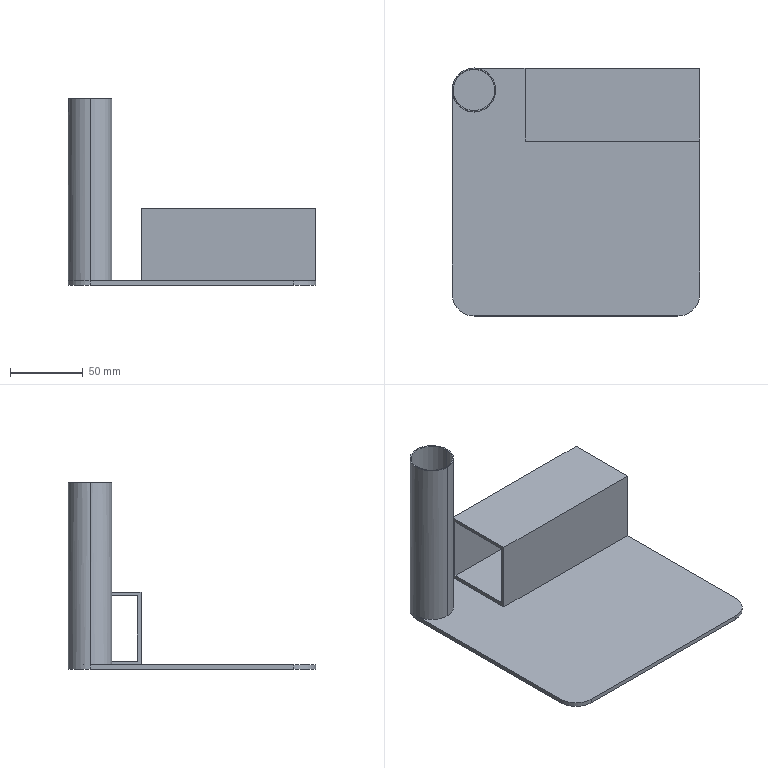Part | STEP file | Component1 | 1 solid | 23 faces | box 170 x 170 x 128 mm | volume 151175 mm3 | plane 16 | cylinder 7 | commonest cylinder face diameters 30 x5 28.6 x2
STEP:
#1=CARTESIAN_POINT('',(29.3,155.,2.));
#2=VERTEX_POINT('',#1);
#3=CARTESIAN_POINT('',(0.7,155.,2.));
#4=VERTEX_POINT('',#3);
#5=CARTESIAN_POINT('',(15.,155.,2.));
#6=DIRECTION('',(0.,0.,1.));
#7=DIRECTION('',(-1.,0.,0.));
#8=AXIS2_PLACEMENT_3D('',#5,#6,#7);
#9=CIRCLE('',#8,14.3);
#10=EDGE_CURVE('',#2,#4,#9,.T.);
#11=ORIENTED_EDGE('',*,*,#10,.F.);
#12=CARTESIAN_POINT('',(29.3,155.,127.));
#13=VERTEX_POINT('',#12);
#14=CARTESIAN_POINT('',(29.3,155.,2.));
#15=DIRECTION('',(0.,0.,1.));
#16=VECTOR('',#15,1000.);
#17=LINE('',#14,#16);
#18=EDGE_CURVE('',#2,#13,#17,.T.);
#19=ORIENTED_EDGE('',*,*,#18,.T.);
#20=CARTESIAN_POINT('',(0.7,155.,127.));
#21=VERTEX_POINT('',#20);
#22=CARTESIAN_POINT('',(15.,155.,127.));
#23=DIRECTION('',(0.,0.,-1.));
#24=DIRECTION('',(-1.,0.,0.));
#25=AXIS2_PLACEMENT_3D('',#22,#23,#24);
#26=CIRCLE('',#25,14.3);
#27=EDGE_CURVE('',#21,#13,#26,.T.);
#28=ORIENTED_EDGE('',*,*,#27,.F.);
#29=CARTESIAN_POINT('',(0.7,155.,2.));
#30=DIRECTION('',(0.,0.,1.));
#31=VECTOR('',#30,1000.);
#32=LINE('',#29,#31);
#33=EDGE_CURVE('',#4,#21,#32,.T.);
#34=ORIENTED_EDGE('',*,*,#33,.F.);
#35=EDGE_LOOP('',(#11,#19,#28,#34));
#36=FACE_OUTER_BOUND('',#35,.T.);
#37=CARTESIAN_POINT('',(15.,155.,2.));
#38=DIRECTION('',(0.,0.,1.));
#39=DIRECTION('',(-1.,0.,0.));
#40=AXIS2_PLACEMENT_3D('',#37,#38,#39);
#41=CYLINDRICAL_SURFACE('',#40,14.3);
#42=ADVANCED_FACE('',(#36),#41,.F.);
#43=CARTESIAN_POINT('',(15.,140.,2.));
#44=VERTEX_POINT('',#43);
#45=CARTESIAN_POINT('',(0.,155.,2.));
#46=VERTEX_POINT('',#45);
#47=CARTESIAN_POINT('',(15.,155.,2.));
#48=DIRECTION('',(0.,0.,-1.));
#49=DIRECTION('',(-1.,0.,0.));
#50=AXIS2_PLACEMENT_3D('',#47,#48,#49);
#51=CIRCLE('',#50,15.);
#52=EDGE_CURVE('',#44,#46,#51,.T.);
#53=ORIENTED_EDGE('',*,*,#52,.F.);
#54=CARTESIAN_POINT('',(15.,140.,127.));
#55=VERTEX_POINT('',#54);
#56=CARTESIAN_POINT('',(15.,140.,0.));
#57=DIRECTION('',(0.,0.,1.));
#58=VECTOR('',#57,1000.);
#59=LINE('',#56,#58);
#60=EDGE_CURVE('',#44,#55,#59,.T.);
#61=ORIENTED_EDGE('',*,*,#60,.T.);
#62=CARTESIAN_POINT('',(15.,170.,127.));
#63=VERTEX_POINT('',#62);
#64=CARTESIAN_POINT('',(15.,155.,127.));
#65=DIRECTION('',(0.,0.,1.));
#66=DIRECTION('',(-1.,0.,0.));
#67=AXIS2_PLACEMENT_3D('',#64,#65,#66);
#68=CIRCLE('',#67,15.);
#69=EDGE_CURVE('',#63,#55,#68,.T.);
#70=ORIENTED_EDGE('',*,*,#69,.F.);
#71=CARTESIAN_POINT('',(15.,170.,2.));
#72=VERTEX_POINT('',#71);
#73=CARTESIAN_POINT('',(15.,170.,0.));
#74=DIRECTION('',(0.,0.,1.));
#75=VECTOR('',#74,1000.);
#76=LINE('',#73,#75);
#77=EDGE_CURVE('',#72,#63,#76,.T.);
#78=ORIENTED_EDGE('',*,*,#77,.F.);
#79=CARTESIAN_POINT('',(15.,170.,-1.));
#80=VERTEX_POINT('',#79);
#81=CARTESIAN_POINT('',(15.,170.,0.));
#82=DIRECTION('',(0.,0.,-1.));
#83=VECTOR('',#82,1000.);
#84=LINE('',#81,#83);
#85=EDGE_CURVE('',#72,#80,#84,.T.);
#86=ORIENTED_EDGE('',*,*,#85,.T.);
#87=CARTESIAN_POINT('',(0.,155.,-1.));
#88=VERTEX_POINT('',#87);
#89=CARTESIAN_POINT('',(15.,155.,-1.));
#90=DIRECTION('',(0.,0.,-1.));
#91=DIRECTION('',(0.,1.,0.));
#92=AXIS2_PLACEMENT_3D('',#89,#90,#91);
#93=CIRCLE('',#92,15.);
#94=EDGE_CURVE('',#88,#80,#93,.T.);
#95=ORIENTED_EDGE('',*,*,#94,.F.);
#96=CARTESIAN_POINT('',(0.,155.,0.));
#97=DIRECTION('',(0.,0.,1.));
#98=VECTOR('',#97,1000.);
#99=LINE('',#96,#98);
#100=EDGE_CURVE('',#88,#46,#99,.T.);
#101=ORIENTED_EDGE('',*,*,#100,.T.);
#102=EDGE_LOOP('',(#53,#61,#70,#78,#86,#95,#101));
#103=FACE_OUTER_BOUND('',#102,.T.);
#104=CARTESIAN_POINT('',(15.,155.,0.));
#105=DIRECTION('',(0.,0.,1.));
#106=DIRECTION('',(0.,1.,0.));
#107=AXIS2_PLACEMENT_3D('',#104,#105,#106);
#108=CYLINDRICAL_SURFACE('',#107,15.);
#109=ADVANCED_FACE('',(#103),#108,.T.);
#110=CARTESIAN_POINT('',(15.,155.,2.));
#111=DIRECTION('',(0.,0.,1.));
#112=DIRECTION('',(-1.,0.,0.));
#113=AXIS2_PLACEMENT_3D('',#110,#111,#112);
#114=CIRCLE('',#113,14.3);
#115=EDGE_CURVE('',#4,#2,#114,.T.);
#116=ORIENTED_EDGE('',*,*,#115,.T.);
#117=ORIENTED_EDGE('',*,*,#10,.T.);
#118=EDGE_LOOP('',(#116,#117));
#119=FACE_OUTER_BOUND('',#118,.T.);
#120=CARTESIAN_POINT('',(85.,85.,2.));
#121=DIRECTION('',(0.,0.,1.));
#122=DIRECTION('',(1.,0.,0.));
#123=AXIS2_PLACEMENT_3D('',#120,#121,#122);
#124=PLANE('',#123);
#125=ADVANCED_FACE('',(#119),#124,.T.);
#126=ORIENTED_EDGE('',*,*,#60,.F.);
#127=CARTESIAN_POINT('',(15.,155.,2.));
#128=DIRECTION('',(0.,0.,-1.));
#129=DIRECTION('',(-1.,0.,0.));
#130=AXIS2_PLACEMENT_3D('',#127,#128,#129);
#131=CIRCLE('',#130,15.);
#132=EDGE_CURVE('',#72,#44,#131,.T.);
#133=ORIENTED_EDGE('',*,*,#132,.F.);
#134=ORIENTED_EDGE('',*,*,#77,.T.);
#135=CARTESIAN_POINT('',(15.,155.,127.));
#136=DIRECTION('',(0.,0.,1.));
#137=DIRECTION('',(-1.,0.,0.));
#138=AXIS2_PLACEMENT_3D('',#135,#136,#137);
#139=CIRCLE('',#138,15.);
#140=EDGE_CURVE('',#55,#63,#139,.T.);
#141=ORIENTED_EDGE('',*,*,#140,.F.);
#142=EDGE_LOOP('',(#126,#133,#134,#141));
#143=FACE_OUTER_BOUND('',#142,.T.);
#144=CARTESIAN_POINT('',(15.,155.,0.));
#145=DIRECTION('',(0.,0.,1.));
#146=DIRECTION('',(0.,1.,0.));
#147=AXIS2_PLACEMENT_3D('',#144,#145,#146);
#148=CYLINDRICAL_SURFACE('',#147,15.);
#149=ADVANCED_FACE('',(#143),#148,.T.);
#150=CARTESIAN_POINT('',(0.,15.,-1.));
#151=VERTEX_POINT('',#150);
#152=CARTESIAN_POINT('',(0.,15.,2.));
#153=VERTEX_POINT('',#152);
#154=CARTESIAN_POINT('',(0.,15.,0.));
#155=DIRECTION('',(0.,0.,1.));
#156=VECTOR('',#155,1000.);
#157=LINE('',#154,#156);
#158=EDGE_CURVE('',#151,#153,#157,.T.);
#159=ORIENTED_EDGE('',*,*,#158,.T.);
#160=CARTESIAN_POINT('',(0.,155.,2.));
#161=DIRECTION('',(0.,-1.,0.));
#162=VECTOR('',#161,1000.);
#163=LINE('',#160,#162);
#164=EDGE_CURVE('',#46,#153,#163,.T.);
#165=ORIENTED_EDGE('',*,*,#164,.F.);
#166=ORIENTED_EDGE('',*,*,#100,.F.);
#167=CARTESIAN_POINT('',(0.,155.,-1.));
#168=DIRECTION('',(0.,1.,0.));
#169=VECTOR('',#168,1000.);
#170=LINE('',#167,#169);
#171=EDGE_CURVE('',#151,#88,#170,.T.);
#172=ORIENTED_EDGE('',*,*,#171,.F.);
#173=EDGE_LOOP('',(#159,#165,#166,#172));
#174=FACE_OUTER_BOUND('',#173,.T.);
#175=CARTESIAN_POINT('',(0.,155.,0.));
#176=DIRECTION('',(-1.,0.,0.));
#177=DIRECTION('',(0.,1.,0.));
#178=AXIS2_PLACEMENT_3D('',#175,#176,#177);
#179=PLANE('',#178);
#180=ADVANCED_FACE('',(#174),#179,.T.);
#181=CARTESIAN_POINT('',(15.,0.,-1.));
#182=VERTEX_POINT('',#181);
#183=CARTESIAN_POINT('',(15.,0.,2.));
#184=VERTEX_POINT('',#183);
#185=CARTESIAN_POINT('',(15.,0.,0.));
#186=DIRECTION('',(0.,0.,1.));
#187=VECTOR('',#186,1000.);
#188=LINE('',#185,#187);
#189=EDGE_CURVE('',#182,#184,#188,.T.);
#190=ORIENTED_EDGE('',*,*,#189,.T.);
#191=CARTESIAN_POINT('',(15.,15.,2.));
#192=DIRECTION('',(0.,0.,1.));
#193=DIRECTION('',(-1.,0.,0.));
#194=AXIS2_PLACEMENT_3D('',#191,#192,#193);
#195=CIRCLE('',#194,15.);
#196=EDGE_CURVE('',#153,#184,#195,.T.);
#197=ORIENTED_EDGE('',*,*,#196,.F.);
#198=ORIENTED_EDGE('',*,*,#158,.F.);
#199=CARTESIAN_POINT('',(15.,15.,-1.));
#200=DIRECTION('',(0.,0.,-1.));
#201=DIRECTION('',(-1.,0.,0.));
#202=AXIS2_PLACEMENT_3D('',#199,#200,#201);
#203=CIRCLE('',#202,15.);
#204=EDGE_CURVE('',#182,#151,#203,.T.);
#205=ORIENTED_EDGE('',*,*,#204,.F.);
#206=EDGE_LOOP('',(#190,#197,#198,#205));
#207=FACE_OUTER_BOUND('',#206,.T.);
#208=CARTESIAN_POINT('',(15.,15.,0.));
#209=DIRECTION('',(0.,0.,1.));
#210=DIRECTION('',(-1.,0.,0.));
#211=AXIS2_PLACEMENT_3D('',#208,#209,#210);
#212=CYLINDRICAL_SURFACE('',#211,15.);
#213=ADVANCED_FACE('',(#207),#212,.T.);
#214=CARTESIAN_POINT('',(155.,0.,-1.));
#215=VERTEX_POINT('',#214);
#216=CARTESIAN_POINT('',(155.,0.,2.));
#217=VERTEX_POINT('',#216);
#218=CARTESIAN_POINT('',(155.,0.,0.));
#219=DIRECTION('',(0.,0.,1.));
#220=VECTOR('',#219,1000.);
#221=LINE('',#218,#220);
#222=EDGE_CURVE('',#215,#217,#221,.T.);
#223=ORIENTED_EDGE('',*,*,#222,.T.);
#224=CARTESIAN_POINT('',(15.,0.,2.));
#225=DIRECTION('',(1.,0.,0.));
#226=VECTOR('',#225,1000.);
#227=LINE('',#224,#226);
#228=EDGE_CURVE('',#184,#217,#227,.T.);
#229=ORIENTED_EDGE('',*,*,#228,.F.);
#230=ORIENTED_EDGE('',*,*,#189,.F.);
#231=CARTESIAN_POINT('',(15.,0.,-1.));
#232=DIRECTION('',(-1.,0.,0.));
#233=VECTOR('',#232,1000.);
#234=LINE('',#231,#233);
#235=EDGE_CURVE('',#215,#182,#234,.T.);
#236=ORIENTED_EDGE('',*,*,#235,.F.);
#237=EDGE_LOOP('',(#223,#229,#230,#236));
#238=FACE_OUTER_BOUND('',#237,.T.);
#239=CARTESIAN_POINT('',(15.,0.,0.));
#240=DIRECTION('',(0.,-1.,0.));
#241=DIRECTION('',(0.,0.,-1.));
#242=AXIS2_PLACEMENT_3D('',#239,#240,#241);
#243=PLANE('',#242);
#244=ADVANCED_FACE('',(#238),#243,.T.);
#245=CARTESIAN_POINT('',(170.,15.,-1.));
#246=VERTEX_POINT('',#245);
#247=CARTESIAN_POINT('',(170.,15.,2.));
#248=VERTEX_POINT('',#247);
#249=CARTESIAN_POINT('',(170.,15.,0.));
#250=DIRECTION('',(0.,0.,1.));
#251=VECTOR('',#250,1000.);
#252=LINE('',#249,#251);
#253=EDGE_CURVE('',#246,#248,#252,.T.);
#254=ORIENTED_EDGE('',*,*,#253,.T.);
#255=CARTESIAN_POINT('',(155.,15.,2.));
#256=DIRECTION('',(0.,0.,1.));
#257=DIRECTION('',(0.,-1.,0.));
#258=AXIS2_PLACEMENT_3D('',#255,#256,#257);
#259=CIRCLE('',#258,15.);
#260=EDGE_CURVE('',#217,#248,#259,.T.);
#261=ORIENTED_EDGE('',*,*,#260,.F.);
#262=ORIENTED_EDGE('',*,*,#222,.F.);
#263=CARTESIAN_POINT('',(155.,15.,-1.));
#264=DIRECTION('',(0.,0.,-1.));
#265=DIRECTION('',(0.,-1.,0.));
#266=AXIS2_PLACEMENT_3D('',#263,#264,#265);
#267=CIRCLE('',#266,15.);
#268=EDGE_CURVE('',#246,#215,#267,.T.);
#269=ORIENTED_EDGE('',*,*,#268,.F.);
#270=EDGE_LOOP('',(#254,#261,#262,#269));
#271=FACE_OUTER_BOUND('',#270,.T.);
#272=CARTESIAN_POINT('',(155.,15.,0.));
#273=DIRECTION('',(0.,0.,1.));
#274=DIRECTION('',(0.,-1.,0.));
#275=AXIS2_PLACEMENT_3D('',#272,#273,#274);
#276=CYLINDRICAL_SURFACE('',#275,15.);
#277=ADVANCED_FACE('',(#271),#276,.T.);
#278=CARTESIAN_POINT('',(170.,122.5,49.5));
#279=VERTEX_POINT('',#278);
#280=CARTESIAN_POINT('',(170.,167.5,49.5));
#281=VERTEX_POINT('',#280);
#282=CARTESIAN_POINT('',(170.,122.5,49.5));
#283=DIRECTION('',(0.,1.,0.));
#284=VECTOR('',#283,1000.);
#285=LINE('',#282,#284);
#286=EDGE_CURVE('',#279,#281,#285,.T.);
#287=ORIENTED_EDGE('',*,*,#286,.T.);
#288=CARTESIAN_POINT('',(170.,167.5,4.5));
#289=VERTEX_POINT('',#288);
#290=CARTESIAN_POINT('',(170.,167.5,49.5));
#291=DIRECTION('',(0.,0.,-1.));
#292=VECTOR('',#291,1000.);
#293=LINE('',#290,#292);
#294=EDGE_CURVE('',#281,#289,#293,.T.);
#295=ORIENTED_EDGE('',*,*,#294,.T.);
#296=CARTESIAN_POINT('',(170.,122.5,4.5));
#297=VERTEX_POINT('',#296);
#298=CARTESIAN_POINT('',(170.,167.5,4.5));
#299=DIRECTION('',(0.,-1.,0.));
#300=VECTOR('',#299,1000.);
#301=LINE('',#298,#300);
#302=EDGE_CURVE('',#289,#297,#301,.T.);
#303=ORIENTED_EDGE('',*,*,#302,.T.);
#304=CARTESIAN_POINT('',(170.,122.5,4.5));
#305=DIRECTION('',(0.,0.,1.));
#306=VECTOR('',#305,1000.);
#307=LINE('',#304,#306);
#308=EDGE_CURVE('',#297,#279,#307,.T.);
#309=ORIENTED_EDGE('',*,*,#308,.T.);
#310=EDGE_LOOP('',(#287,#295,#303,#309));
#311=FACE_BOUND('',#310,.T.);
#312=CARTESIAN_POINT('',(170.,155.,-1.));
#313=VERTEX_POINT('',#312);
#314=CARTESIAN_POINT('',(170.,155.,2.));
#315=VERTEX_POINT('',#314);
#316=CARTESIAN_POINT('',(170.,155.,0.));
#317=DIRECTION('',(0.,0.,1.));
#318=VECTOR('',#317,1000.);
#319=LINE('',#316,#318);
#320=EDGE_CURVE('',#313,#315,#319,.T.);
#321=ORIENTED_EDGE('',*,*,#320,.T.);
#322=CARTESIAN_POINT('',(170.,170.,2.));
#323=VERTEX_POINT('',#322);
#324=CARTESIAN_POINT('',(170.,170.,2.));
#325=DIRECTION('',(0.,-1.,0.));
#326=VECTOR('',#325,1000.);
#327=LINE('',#324,#326);
#328=EDGE_CURVE('',#323,#315,#327,.T.);
#329=ORIENTED_EDGE('',*,*,#328,.F.);
#330=CARTESIAN_POINT('',(170.,170.,52.));
#331=VERTEX_POINT('',#330);
#332=CARTESIAN_POINT('',(170.,170.,52.));
#333=DIRECTION('',(0.,0.,-1.));
#334=VECTOR('',#333,1000.);
#335=LINE('',#332,#334);
#336=EDGE_CURVE('',#331,#323,#335,.T.);
#337=ORIENTED_EDGE('',*,*,#336,.F.);
#338=CARTESIAN_POINT('',(170.,120.,52.));
#339=VERTEX_POINT('',#338);
#340=CARTESIAN_POINT('',(170.,120.,52.));
#341=DIRECTION('',(0.,1.,0.));
#342=VECTOR('',#341,1000.);
#343=LINE('',#340,#342);
#344=EDGE_CURVE('',#339,#331,#343,.T.);
#345=ORIENTED_EDGE('',*,*,#344,.F.);
#346=CARTESIAN_POINT('',(170.,120.,2.));
#347=VERTEX_POINT('',#346);
#348=CARTESIAN_POINT('',(170.,120.,2.));
#349=DIRECTION('',(0.,0.,1.));
#350=VECTOR('',#349,1000.);
#351=LINE('',#348,#350);
#352=EDGE_CURVE('',#347,#339,#351,.T.);
#353=ORIENTED_EDGE('',*,*,#352,.F.);
#354=CARTESIAN_POINT('',(170.,15.,2.));
#355=DIRECTION('',(0.,1.,0.));
#356=VECTOR('',#355,1000.);
#357=LINE('',#354,#356);
#358=EDGE_CURVE('',#248,#347,#357,.T.);
#359=ORIENTED_EDGE('',*,*,#358,.F.);
#360=ORIENTED_EDGE('',*,*,#253,.F.);
#361=CARTESIAN_POINT('',(170.,15.,-1.));
#362=DIRECTION('',(0.,-1.,0.));
#363=VECTOR('',#362,1000.);
#364=LINE('',#361,#363);
#365=EDGE_CURVE('',#313,#246,#364,.T.);
#366=ORIENTED_EDGE('',*,*,#365,.F.);
#367=EDGE_LOOP('',(#321,#329,#337,#345,#353,#359,#360,#366));
#368=FACE_OUTER_BOUND('',#367,.T.);
#369=CARTESIAN_POINT('',(170.,15.,0.));
#370=DIRECTION('',(1.,0.,0.));
#371=DIRECTION('',(0.,1.,0.));
#372=AXIS2_PLACEMENT_3D('',#369,#370,#371);
#373=PLANE('',#372);
#374=ADVANCED_FACE('',(#311,#368),#373,.T.);
#375=CARTESIAN_POINT('',(155.,170.,-1.));
#376=VERTEX_POINT('',#375);
#377=CARTESIAN_POINT('',(155.,170.,2.));
#378=VERTEX_POINT('',#377);
#379=CARTESIAN_POINT('',(155.,170.,0.));
#380=DIRECTION('',(0.,0.,1.));
#381=VECTOR('',#380,1000.);
#382=LINE('',#379,#381);
#383=EDGE_CURVE('',#376,#378,#382,.T.);
#384=ORIENTED_EDGE('',*,*,#383,.T.);
#385=CARTESIAN_POINT('',(155.,155.,2.));
#386=DIRECTION('',(0.,0.,1.));
#387=DIRECTION('',(1.,0.,0.));
#388=AXIS2_PLACEMENT_3D('',#385,#386,#387);
#389=CIRCLE('',#388,15.);
#390=EDGE_CURVE('',#315,#378,#389,.T.);
#391=ORIENTED_EDGE('',*,*,#390,.F.);
#392=ORIENTED_EDGE('',*,*,#320,.F.);
#393=CARTESIAN_POINT('',(155.,155.,-1.));
#394=DIRECTION('',(0.,0.,-1.));
#395=DIRECTION('',(1.,0.,0.));
#396=AXIS2_PLACEMENT_3D('',#393,#394,#395);
#397=CIRCLE('',#396,15.);
#398=EDGE_CURVE('',#376,#313,#397,.T.);
#399=ORIENTED_EDGE('',*,*,#398,.F.);
#400=EDGE_LOOP('',(#384,#391,#392,#399));
#401=FACE_OUTER_BOUND('',#400,.T.);
#402=CARTESIAN_POINT('',(155.,155.,0.));
#403=DIRECTION('',(0.,0.,1.));
#404=DIRECTION('',(1.,0.,0.));
#405=AXIS2_PLACEMENT_3D('',#402,#403,#404);
#406=CYLINDRICAL_SURFACE('',#405,15.);
#407=ADVANCED_FACE('',(#401),#406,.T.);
#408=ORIENTED_EDGE('',*,*,#85,.F.);
#409=CARTESIAN_POINT('',(50.,170.,2.));
#410=VERTEX_POINT('',#409);
#411=CARTESIAN_POINT('',(155.,170.,2.));
#412=DIRECTION('',(-1.,0.,0.));
#413=VECTOR('',#412,1000.);
#414=LINE('',#411,#413);
#415=EDGE_CURVE('',#410,#72,#414,.T.);
#416=ORIENTED_EDGE('',*,*,#415,.F.);
#417=CARTESIAN_POINT('',(50.,170.,52.));
#418=VERTEX_POINT('',#417);
#419=CARTESIAN_POINT('',(50.,170.,52.));
#420=DIRECTION('',(0.,0.,-1.));
#421=VECTOR('',#420,1000.);
#422=LINE('',#419,#421);
#423=EDGE_CURVE('',#418,#410,#422,.T.);
#424=ORIENTED_EDGE('',*,*,#423,.F.);
#425=CARTESIAN_POINT('',(170.,170.,52.));
#426=DIRECTION('',(-1.,0.,0.));
#427=VECTOR('',#426,1000.);
#428=LINE('',#425,#427);
#429=EDGE_CURVE('',#331,#418,#428,.T.);
#430=ORIENTED_EDGE('',*,*,#429,.F.);
#431=ORIENTED_EDGE('',*,*,#336,.T.);
#432=CARTESIAN_POINT('',(170.,170.,2.));
#433=DIRECTION('',(-1.,0.,0.));
#434=VECTOR('',#433,1000.);
#435=LINE('',#432,#434);
#436=EDGE_CURVE('',#323,#378,#435,.T.);
#437=ORIENTED_EDGE('',*,*,#436,.T.);
#438=ORIENTED_EDGE('',*,*,#383,.F.);
#439=CARTESIAN_POINT('',(155.,170.,-1.));
#440=DIRECTION('',(1.,0.,0.));
#441=VECTOR('',#440,1000.);
#442=LINE('',#439,#441);
#443=EDGE_CURVE('',#80,#376,#442,.T.);
#444=ORIENTED_EDGE('',*,*,#443,.F.);
#445=EDGE_LOOP('',(#408,#416,#424,#430,#431,#437,#438,#444));
#446=FACE_OUTER_BOUND('',#445,.T.);
#447=CARTESIAN_POINT('',(155.,170.,0.));
#448=DIRECTION('',(0.,1.,0.));
#449=DIRECTION('',(1.,0.,0.));
#450=AXIS2_PLACEMENT_3D('',#447,#448,#449);
#451=PLANE('',#450);
#452=ADVANCED_FACE('',(#446),#451,.T.);
#453=ORIENTED_EDGE('',*,*,#27,.T.);
#454=CARTESIAN_POINT('',(15.,155.,127.));
#455=DIRECTION('',(0.,0.,-1.));
#456=DIRECTION('',(-1.,0.,0.));
#457=AXIS2_PLACEMENT_3D('',#454,#455,#456);
#458=CIRCLE('',#457,14.3);
#459=EDGE_CURVE('',#13,#21,#458,.T.);
#460=ORIENTED_EDGE('',*,*,#459,.T.);
#461=EDGE_LOOP('',(#453,#460));
#462=FACE_BOUND('',#461,.T.);
#463=ORIENTED_EDGE('',*,*,#69,.T.);
#464=ORIENTED_EDGE('',*,*,#140,.T.);
#465=EDGE_LOOP('',(#463,#464));
#466=FACE_OUTER_BOUND('',#465,.T.);
#467=CARTESIAN_POINT('',(15.,155.,127.));
#468=DIRECTION('',(0.,0.,1.));
#469=DIRECTION('',(1.,0.,0.));
#470=AXIS2_PLACEMENT_3D('',#467,#468,#469);
#471=PLANE('',#470);
#472=ADVANCED_FACE('',(#462,#466),#471,.T.);
#473=ORIENTED_EDGE('',*,*,#18,.F.);
#474=ORIENTED_EDGE('',*,*,#115,.F.);
#475=ORIENTED_EDGE('',*,*,#33,.T.);
#476=ORIENTED_EDGE('',*,*,#459,.F.);
#477=EDGE_LOOP('',(#473,#474,#475,#476));
#478=FACE_OUTER_BOUND('',#477,.T.);
#479=CARTESIAN_POINT('',(15.,155.,2.));
#480=DIRECTION('',(0.,0.,1.));
#481=DIRECTION('',(-1.,0.,0.));
#482=AXIS2_PLACEMENT_3D('',#479,#480,#481);
#483=CYLINDRICAL_SURFACE('',#482,14.3);
#484=ADVANCED_FACE('',(#478),#483,.F.);
#485=ORIENTED_EDGE('',*,*,#94,.T.);
#486=ORIENTED_EDGE('',*,*,#443,.T.);
#487=ORIENTED_EDGE('',*,*,#398,.T.);
#488=ORIENTED_EDGE('',*,*,#365,.T.);
#489=ORIENTED_EDGE('',*,*,#268,.T.);
#490=ORIENTED_EDGE('',*,*,#235,.T.);
#491=ORIENTED_EDGE('',*,*,#204,.T.);
#492=ORIENTED_EDGE('',*,*,#171,.T.);
#493=EDGE_LOOP('',(#485,#486,#487,#488,#489,#490,#491,#492));
#494=FACE_OUTER_BOUND('',#493,.T.);
#495=CARTESIAN_POINT('',(85.,85.,-1.));
#496=DIRECTION('',(0.,0.,1.));
#497=DIRECTION('',(1.,0.,0.));
#498=AXIS2_PLACEMENT_3D('',#495,#496,#497);
#499=PLANE('',#498);
#500=ADVANCED_FACE('',(#494),#499,.F.);
#501=CARTESIAN_POINT('',(50.,120.,2.));
#502=VERTEX_POINT('',#501);
#503=CARTESIAN_POINT('',(127.5,120.,2.));
#504=DIRECTION('',(-1.,0.,0.));
#505=VECTOR('',#504,1000.);
#506=LINE('',#503,#505);
#507=EDGE_CURVE('',#347,#502,#506,.T.);
#508=ORIENTED_EDGE('',*,*,#507,.T.);
#509=CARTESIAN_POINT('',(50.,115.,2.));
#510=DIRECTION('',(0.,1.,0.));
#511=VECTOR('',#510,1000.);
#512=LINE('',#509,#511);
#513=EDGE_CURVE('',#502,#410,#512,.T.);
#514=ORIENTED_EDGE('',*,*,#513,.T.);
#515=ORIENTED_EDGE('',*,*,#415,.T.);
#516=ORIENTED_EDGE('',*,*,#132,.T.);
#517=ORIENTED_EDGE('',*,*,#52,.T.);
#518=ORIENTED_EDGE('',*,*,#164,.T.);
#519=ORIENTED_EDGE('',*,*,#196,.T.);
#520=ORIENTED_EDGE('',*,*,#228,.T.);
#521=ORIENTED_EDGE('',*,*,#260,.T.);
#522=ORIENTED_EDGE('',*,*,#358,.T.);
#523=EDGE_LOOP('',(#508,#514,#515,#516,#517,#518,#519,#520,#521,#522));
#524=FACE_OUTER_BOUND('',#523,.T.);
#525=CARTESIAN_POINT('',(85.,85.,2.));
#526=DIRECTION('',(0.,0.,1.));
#527=DIRECTION('',(1.,0.,0.));
#528=AXIS2_PLACEMENT_3D('',#525,#526,#527);
#529=PLANE('',#528);
#530=ADVANCED_FACE('',(#524),#529,.T.);
#531=CARTESIAN_POINT('',(50.,167.5,49.5));
#532=VERTEX_POINT('',#531);
#533=CARTESIAN_POINT('',(50.,122.5,49.5));
#534=VERTEX_POINT('',#533);
#535=CARTESIAN_POINT('',(50.,122.5,49.5));
#536=DIRECTION('',(0.,-1.,0.));
#537=VECTOR('',#536,1000.);
#538=LINE('',#535,#537);
#539=EDGE_CURVE('',#532,#534,#538,.T.);
#540=ORIENTED_EDGE('',*,*,#539,.T.);
#541=CARTESIAN_POINT('',(50.,122.5,4.5));
#542=VERTEX_POINT('',#541);
#543=CARTESIAN_POINT('',(50.,122.5,4.5));
#544=DIRECTION('',(0.,0.,-1.));
#545=VECTOR('',#544,1000.);
#546=LINE('',#543,#545);
#547=EDGE_CURVE('',#534,#542,#546,.T.);
#548=ORIENTED_EDGE('',*,*,#547,.T.);
#549=CARTESIAN_POINT('',(50.,167.5,4.5));
#550=VERTEX_POINT('',#549);
#551=CARTESIAN_POINT('',(50.,167.5,4.5));
#552=DIRECTION('',(0.,1.,0.));
#553=VECTOR('',#552,1000.);
#554=LINE('',#551,#553);
#555=EDGE_CURVE('',#542,#550,#554,.T.);
#556=ORIENTED_EDGE('',*,*,#555,.T.);
#557=CARTESIAN_POINT('',(50.,167.5,49.5));
#558=DIRECTION('',(0.,0.,1.));
#559=VECTOR('',#558,1000.);
#560=LINE('',#557,#559);
#561=EDGE_CURVE('',#550,#532,#560,.T.);
#562=ORIENTED_EDGE('',*,*,#561,.T.);
#563=EDGE_LOOP('',(#540,#548,#556,#562));
#564=FACE_BOUND('',#563,.T.);
#565=CARTESIAN_POINT('',(50.,120.,52.));
#566=VERTEX_POINT('',#565);
#567=CARTESIAN_POINT('',(50.,120.,52.));
#568=DIRECTION('',(0.,1.,0.));
#569=VECTOR('',#568,1000.);
#570=LINE('',#567,#569);
#571=EDGE_CURVE('',#566,#418,#570,.T.);
#572=ORIENTED_EDGE('',*,*,#571,.T.);
#573=ORIENTED_EDGE('',*,*,#423,.T.);
#574=ORIENTED_EDGE('',*,*,#513,.F.);
#575=CARTESIAN_POINT('',(50.,120.,2.));
#576=DIRECTION('',(0.,0.,1.));
#577=VECTOR('',#576,1000.);
#578=LINE('',#575,#577);
#579=EDGE_CURVE('',#502,#566,#578,.T.);
#580=ORIENTED_EDGE('',*,*,#579,.T.);
#581=EDGE_LOOP('',(#572,#573,#574,#580));
#582=FACE_OUTER_BOUND('',#581,.T.);
#583=CARTESIAN_POINT('',(50.,145.,27.));
#584=DIRECTION('',(-1.,0.,0.));
#585=DIRECTION('',(0.,0.,1.));
#586=AXIS2_PLACEMENT_3D('',#583,#584,#585);
#587=PLANE('',#586);
#588=ADVANCED_FACE('',(#564,#582),#587,.T.);
#589=ORIENTED_EDGE('',*,*,#344,.T.);
#590=ORIENTED_EDGE('',*,*,#429,.T.);
#591=ORIENTED_EDGE('',*,*,#571,.F.);
#592=CARTESIAN_POINT('',(170.,120.,52.));
#593=DIRECTION('',(-1.,0.,0.));
#594=VECTOR('',#593,1000.);
#595=LINE('',#592,#594);
#596=EDGE_CURVE('',#339,#566,#595,.T.);
#597=ORIENTED_EDGE('',*,*,#596,.F.);
#598=EDGE_LOOP('',(#589,#590,#591,#597));
#599=FACE_OUTER_BOUND('',#598,.T.);
#600=CARTESIAN_POINT('',(170.,120.,52.));
#601=DIRECTION('',(0.,0.,1.));
#602=DIRECTION('',(1.,0.,0.));
#603=AXIS2_PLACEMENT_3D('',#600,#601,#602);
#604=PLANE('',#603);
#605=ADVANCED_FACE('',(#599),#604,.T.);
#606=ORIENTED_EDGE('',*,*,#352,.T.);
#607=ORIENTED_EDGE('',*,*,#596,.T.);
#608=ORIENTED_EDGE('',*,*,#579,.F.);
#609=ORIENTED_EDGE('',*,*,#507,.F.);
#610=EDGE_LOOP('',(#606,#607,#608,#609));
#611=FACE_OUTER_BOUND('',#610,.T.);
#612=CARTESIAN_POINT('',(170.,120.,2.));
#613=DIRECTION('',(0.,-1.,0.));
#614=DIRECTION('',(0.,0.,-1.));
#615=AXIS2_PLACEMENT_3D('',#612,#613,#614);
#616=PLANE('',#615);
#617=ADVANCED_FACE('',(#611),#616,.T.);
#618=ORIENTED_EDGE('',*,*,#286,.F.);
#619=CARTESIAN_POINT('',(170.,122.5,49.5));
#620=DIRECTION('',(-1.,0.,0.));
#621=VECTOR('',#620,1000.);
#622=LINE('',#619,#621);
#623=EDGE_CURVE('',#279,#534,#622,.T.);
#624=ORIENTED_EDGE('',*,*,#623,.T.);
#625=ORIENTED_EDGE('',*,*,#539,.F.);
#626=CARTESIAN_POINT('',(170.,167.5,49.5));
#627=DIRECTION('',(-1.,0.,0.));
#628=VECTOR('',#627,1000.);
#629=LINE('',#626,#628);
#630=EDGE_CURVE('',#281,#532,#629,.T.);
#631=ORIENTED_EDGE('',*,*,#630,.F.);
#632=EDGE_LOOP('',(#618,#624,#625,#631));
#633=FACE_OUTER_BOUND('',#632,.T.);
#634=CARTESIAN_POINT('',(170.,167.5,49.5));
#635=DIRECTION('',(0.,0.,-1.));
#636=DIRECTION('',(0.,-1.,0.));
#637=AXIS2_PLACEMENT_3D('',#634,#635,#636);
#638=PLANE('',#637);
#639=ADVANCED_FACE('',(#633),#638,.T.);
#640=ORIENTED_EDGE('',*,*,#308,.F.);
#641=CARTESIAN_POINT('',(170.,122.5,4.5));
#642=DIRECTION('',(-1.,0.,0.));
#643=VECTOR('',#642,1000.);
#644=LINE('',#641,#643);
#645=EDGE_CURVE('',#297,#542,#644,.T.);
#646=ORIENTED_EDGE('',*,*,#645,.T.);
#647=ORIENTED_EDGE('',*,*,#547,.F.);
#648=ORIENTED_EDGE('',*,*,#623,.F.);
#649=EDGE_LOOP('',(#640,#646,#647,#648));
#650=FACE_OUTER_BOUND('',#649,.T.);
#651=CARTESIAN_POINT('',(170.,122.5,49.5));
#652=DIRECTION('',(0.,1.,0.));
#653=DIRECTION('',(1.,0.,0.));
#654=AXIS2_PLACEMENT_3D('',#651,#652,#653);
#655=PLANE('',#654);
#656=ADVANCED_FACE('',(#650),#655,.T.);
#657=ORIENTED_EDGE('',*,*,#302,.F.);
#658=CARTESIAN_POINT('',(170.,167.5,4.5));
#659=DIRECTION('',(-1.,0.,0.));
#660=VECTOR('',#659,1000.);
#661=LINE('',#658,#660);
#662=EDGE_CURVE('',#289,#550,#661,.T.);
#663=ORIENTED_EDGE('',*,*,#662,.T.);
#664=ORIENTED_EDGE('',*,*,#555,.F.);
#665=ORIENTED_EDGE('',*,*,#645,.F.);
#666=EDGE_LOOP('',(#657,#663,#664,#665));
#667=FACE_OUTER_BOUND('',#666,.T.);
#668=CARTESIAN_POINT('',(170.,122.5,4.5));
#669=DIRECTION('',(0.,0.,1.));
#670=DIRECTION('',(1.,0.,0.));
#671=AXIS2_PLACEMENT_3D('',#668,#669,#670);
#672=PLANE('',#671);
#673=ADVANCED_FACE('',(#667),#672,.T.);
#674=ORIENTED_EDGE('',*,*,#294,.F.);
#675=ORIENTED_EDGE('',*,*,#630,.T.);
#676=ORIENTED_EDGE('',*,*,#561,.F.);
#677=ORIENTED_EDGE('',*,*,#662,.F.);
#678=EDGE_LOOP('',(#674,#675,#676,#677));
#679=FACE_OUTER_BOUND('',#678,.T.);
#680=CARTESIAN_POINT('',(170.,167.5,4.5));
#681=DIRECTION('',(0.,-1.,0.));
#682=DIRECTION('',(0.,0.,-1.));
#683=AXIS2_PLACEMENT_3D('',#680,#681,#682);
#684=PLANE('',#683);
#685=ADVANCED_FACE('',(#679),#684,.T.);
#686=ORIENTED_EDGE('',*,*,#390,.T.);
#687=ORIENTED_EDGE('',*,*,#436,.F.);
#688=ORIENTED_EDGE('',*,*,#328,.T.);
#689=EDGE_LOOP('',(#686,#687,#688));
#690=FACE_OUTER_BOUND('',#689,.T.);
#691=CARTESIAN_POINT('',(170.,170.,2.));
#692=DIRECTION('',(0.,0.,-1.));
#693=DIRECTION('',(0.,-1.,0.));
#694=AXIS2_PLACEMENT_3D('',#691,#692,#693);
#695=PLANE('',#694);
#696=ADVANCED_FACE('',(#690),#695,.T.);
#697=CLOSED_SHELL('',(#42,#109,#125,#149,#180,#213,#244,#277,#374,#407,#452,#472,#484,#500,#530,#588,#605,#617,#639,#656,#673,#685,#696));
#698=MANIFOLD_SOLID_BREP('',#697);
#699=CARTESIAN_POINT('',(0.,0.,0.));
#700=DIRECTION('',(0.,0.,1.));
#701=DIRECTION('',(1.,0.,0.));
#702=AXIS2_PLACEMENT_3D('',#699,#700,#701);
#703=(LENGTH_UNIT()NAMED_UNIT(*)SI_UNIT(.MILLI.,.METRE.));
#704=UNCERTAINTY_MEASURE_WITH_UNIT(LENGTH_MEASURE(0.00001),#703,'','');
#705=(NAMED_UNIT(*)PLANE_ANGLE_UNIT()SI_UNIT($,.RADIAN.));
#706=(NAMED_UNIT(*)SI_UNIT($,.STERADIAN.)SOLID_ANGLE_UNIT());
#707=(GEOMETRIC_REPRESENTATION_CONTEXT(3)GLOBAL_UNCERTAINTY_ASSIGNED_CONTEXT((#704))GLOBAL_UNIT_ASSIGNED_CONTEXT((#703,#705,#706))REPRESENTATION_CONTEXT('',''));
#708=ADVANCED_BREP_SHAPE_REPRESENTATION('',(#698,#702),#707);